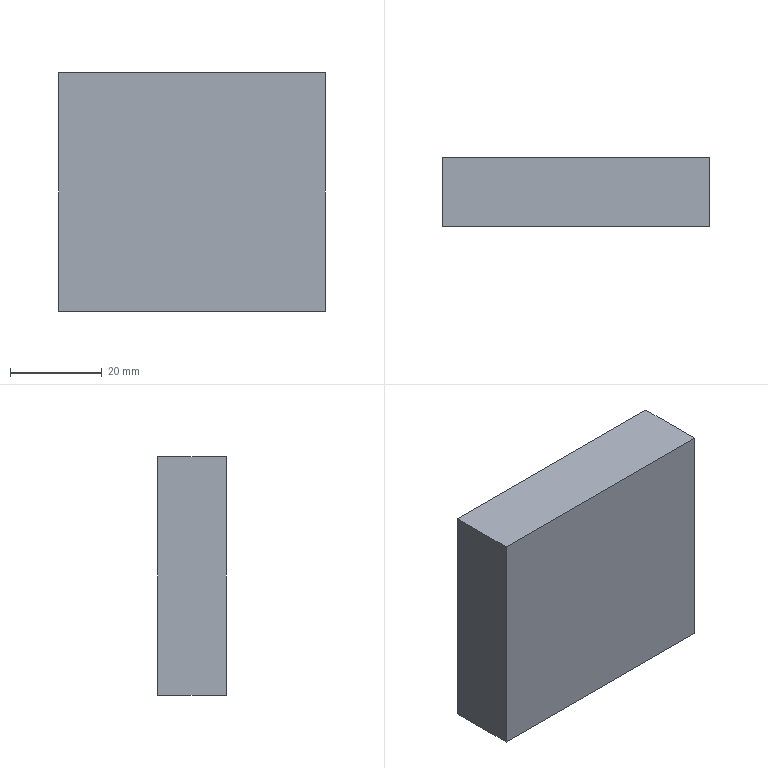Part | SolidWorks | features FlatPattern 1, SMBaseFlange 1, SheetMetal 1 | 1 solid | 6 faces | box 58 x 15 x 52 mm | volume 45240 mm3 | plane 6
STEP:
#1=CARTESIAN_POINT('',(0.,0.,0.));
#2=VERTEX_POINT('',#1);
#3=CARTESIAN_POINT('',(0.,0.,52.));
#4=VERTEX_POINT('',#3);
#5=CARTESIAN_POINT('',(0.,0.,0.));
#6=DIRECTION('',(0.,0.,1.));
#7=VECTOR('',#6,1000.);
#8=LINE('',#5,#7);
#9=EDGE_CURVE('',#2,#4,#8,.T.);
#10=ORIENTED_EDGE('',*,*,#9,.F.);
#11=CARTESIAN_POINT('',(0.,-15.,0.));
#12=VERTEX_POINT('',#11);
#13=CARTESIAN_POINT('',(0.,-15.,0.));
#14=DIRECTION('',(0.,1.,0.));
#15=VECTOR('',#14,1000.);
#16=LINE('',#13,#15);
#17=EDGE_CURVE('',#12,#2,#16,.T.);
#18=ORIENTED_EDGE('',*,*,#17,.F.);
#19=CARTESIAN_POINT('',(0.,-15.,52.));
#20=VERTEX_POINT('',#19);
#21=CARTESIAN_POINT('',(0.,-15.,0.));
#22=DIRECTION('',(0.,0.,1.));
#23=VECTOR('',#22,1000.);
#24=LINE('',#21,#23);
#25=EDGE_CURVE('',#12,#20,#24,.T.);
#26=ORIENTED_EDGE('',*,*,#25,.T.);
#27=CARTESIAN_POINT('',(0.,-15.,52.));
#28=DIRECTION('',(0.,1.,0.));
#29=VECTOR('',#28,1000.);
#30=LINE('',#27,#29);
#31=EDGE_CURVE('',#20,#4,#30,.T.);
#32=ORIENTED_EDGE('',*,*,#31,.T.);
#33=EDGE_LOOP('',(#10,#18,#26,#32));
#34=FACE_OUTER_BOUND('',#33,.T.);
#35=CARTESIAN_POINT('',(0.,-15.,0.));
#36=DIRECTION('',(-1.,0.,0.));
#37=DIRECTION('',(0.,0.,1.));
#38=AXIS2_PLACEMENT_3D('',#35,#36,#37);
#39=PLANE('',#38);
#40=ADVANCED_FACE('',(#34),#39,.T.);
#41=CARTESIAN_POINT('',(58.,0.,0.));
#42=VERTEX_POINT('',#41);
#43=CARTESIAN_POINT('',(0.,0.,0.));
#44=DIRECTION('',(-1.,0.,0.));
#45=VECTOR('',#44,1000.);
#46=LINE('',#43,#45);
#47=EDGE_CURVE('',#42,#2,#46,.T.);
#48=ORIENTED_EDGE('',*,*,#47,.F.);
#49=CARTESIAN_POINT('',(58.,-15.,0.));
#50=VERTEX_POINT('',#49);
#51=CARTESIAN_POINT('',(58.,-15.,0.));
#52=DIRECTION('',(0.,1.,0.));
#53=VECTOR('',#52,1000.);
#54=LINE('',#51,#53);
#55=EDGE_CURVE('',#50,#42,#54,.T.);
#56=ORIENTED_EDGE('',*,*,#55,.F.);
#57=CARTESIAN_POINT('',(0.,-15.,0.));
#58=DIRECTION('',(-1.,0.,0.));
#59=VECTOR('',#58,1000.);
#60=LINE('',#57,#59);
#61=EDGE_CURVE('',#50,#12,#60,.T.);
#62=ORIENTED_EDGE('',*,*,#61,.T.);
#63=ORIENTED_EDGE('',*,*,#17,.T.);
#64=EDGE_LOOP('',(#48,#56,#62,#63));
#65=FACE_OUTER_BOUND('',#64,.T.);
#66=CARTESIAN_POINT('',(0.,-15.,0.));
#67=DIRECTION('',(0.,0.,-1.));
#68=DIRECTION('',(-1.,0.,0.));
#69=AXIS2_PLACEMENT_3D('',#66,#67,#68);
#70=PLANE('',#69);
#71=ADVANCED_FACE('',(#65),#70,.T.);
#72=CARTESIAN_POINT('',(58.,0.,52.));
#73=VERTEX_POINT('',#72);
#74=CARTESIAN_POINT('',(58.,0.,0.));
#75=DIRECTION('',(0.,0.,-1.));
#76=VECTOR('',#75,1000.);
#77=LINE('',#74,#76);
#78=EDGE_CURVE('',#73,#42,#77,.T.);
#79=ORIENTED_EDGE('',*,*,#78,.F.);
#80=CARTESIAN_POINT('',(58.,-15.,52.));
#81=VERTEX_POINT('',#80);
#82=CARTESIAN_POINT('',(58.,-15.,52.));
#83=DIRECTION('',(0.,1.,0.));
#84=VECTOR('',#83,1000.);
#85=LINE('',#82,#84);
#86=EDGE_CURVE('',#81,#73,#85,.T.);
#87=ORIENTED_EDGE('',*,*,#86,.F.);
#88=CARTESIAN_POINT('',(58.,-15.,0.));
#89=DIRECTION('',(0.,0.,-1.));
#90=VECTOR('',#89,1000.);
#91=LINE('',#88,#90);
#92=EDGE_CURVE('',#81,#50,#91,.T.);
#93=ORIENTED_EDGE('',*,*,#92,.T.);
#94=ORIENTED_EDGE('',*,*,#55,.T.);
#95=EDGE_LOOP('',(#79,#87,#93,#94));
#96=FACE_OUTER_BOUND('',#95,.T.);
#97=CARTESIAN_POINT('',(58.,-15.,0.));
#98=DIRECTION('',(1.,0.,0.));
#99=DIRECTION('',(0.,0.,-1.));
#100=AXIS2_PLACEMENT_3D('',#97,#98,#99);
#101=PLANE('',#100);
#102=ADVANCED_FACE('',(#96),#101,.T.);
#103=CARTESIAN_POINT('',(0.,0.,52.));
#104=DIRECTION('',(1.,0.,0.));
#105=VECTOR('',#104,1000.);
#106=LINE('',#103,#105);
#107=EDGE_CURVE('',#4,#73,#106,.T.);
#108=ORIENTED_EDGE('',*,*,#107,.F.);
#109=ORIENTED_EDGE('',*,*,#31,.F.);
#110=CARTESIAN_POINT('',(0.,-15.,52.));
#111=DIRECTION('',(1.,0.,0.));
#112=VECTOR('',#111,1000.);
#113=LINE('',#110,#112);
#114=EDGE_CURVE('',#20,#81,#113,.T.);
#115=ORIENTED_EDGE('',*,*,#114,.T.);
#116=ORIENTED_EDGE('',*,*,#86,.T.);
#117=EDGE_LOOP('',(#108,#109,#115,#116));
#118=FACE_OUTER_BOUND('',#117,.T.);
#119=CARTESIAN_POINT('',(0.,-15.,52.));
#120=DIRECTION('',(0.,0.,1.));
#121=DIRECTION('',(1.,0.,0.));
#122=AXIS2_PLACEMENT_3D('',#119,#120,#121);
#123=PLANE('',#122);
#124=ADVANCED_FACE('',(#118),#123,.T.);
#125=ORIENTED_EDGE('',*,*,#25,.F.);
#126=ORIENTED_EDGE('',*,*,#61,.F.);
#127=ORIENTED_EDGE('',*,*,#92,.F.);
#128=ORIENTED_EDGE('',*,*,#114,.F.);
#129=EDGE_LOOP('',(#125,#126,#127,#128));
#130=FACE_OUTER_BOUND('',#129,.T.);
#131=CARTESIAN_POINT('',(0.,-15.,0.));
#132=DIRECTION('',(0.,1.,0.));
#133=DIRECTION('',(0.,0.,1.));
#134=AXIS2_PLACEMENT_3D('',#131,#132,#133);
#135=PLANE('',#134);
#136=ADVANCED_FACE('',(#130),#135,.F.);
#137=ORIENTED_EDGE('',*,*,#9,.T.);
#138=ORIENTED_EDGE('',*,*,#107,.T.);
#139=ORIENTED_EDGE('',*,*,#78,.T.);
#140=ORIENTED_EDGE('',*,*,#47,.T.);
#141=EDGE_LOOP('',(#137,#138,#139,#140));
#142=FACE_OUTER_BOUND('',#141,.T.);
#143=CARTESIAN_POINT('',(0.,0.,0.));
#144=DIRECTION('',(0.,1.,0.));
#145=DIRECTION('',(0.,0.,1.));
#146=AXIS2_PLACEMENT_3D('',#143,#144,#145);
#147=PLANE('',#146);
#148=ADVANCED_FACE('',(#142),#147,.T.);
#149=CLOSED_SHELL('',(#40,#71,#102,#124,#136,#148));
#150=MANIFOLD_SOLID_BREP('',#149);
#151=CARTESIAN_POINT('',(0.,0.,0.));
#152=DIRECTION('',(0.,0.,1.));
#153=DIRECTION('',(1.,0.,0.));
#154=AXIS2_PLACEMENT_3D('',#151,#152,#153);
#155=(LENGTH_UNIT()NAMED_UNIT(*)SI_UNIT(.MILLI.,.METRE.));
#156=UNCERTAINTY_MEASURE_WITH_UNIT(LENGTH_MEASURE(0.00001),#155,'','');
#157=(NAMED_UNIT(*)PLANE_ANGLE_UNIT()SI_UNIT($,.RADIAN.));
#158=(NAMED_UNIT(*)SI_UNIT($,.STERADIAN.)SOLID_ANGLE_UNIT());
#159=(GEOMETRIC_REPRESENTATION_CONTEXT(3)GLOBAL_UNCERTAINTY_ASSIGNED_CONTEXT((#156))GLOBAL_UNIT_ASSIGNED_CONTEXT((#155,#157,#158))REPRESENTATION_CONTEXT('',''));
#160=ADVANCED_BREP_SHAPE_REPRESENTATION('',(#150,#154),#159);